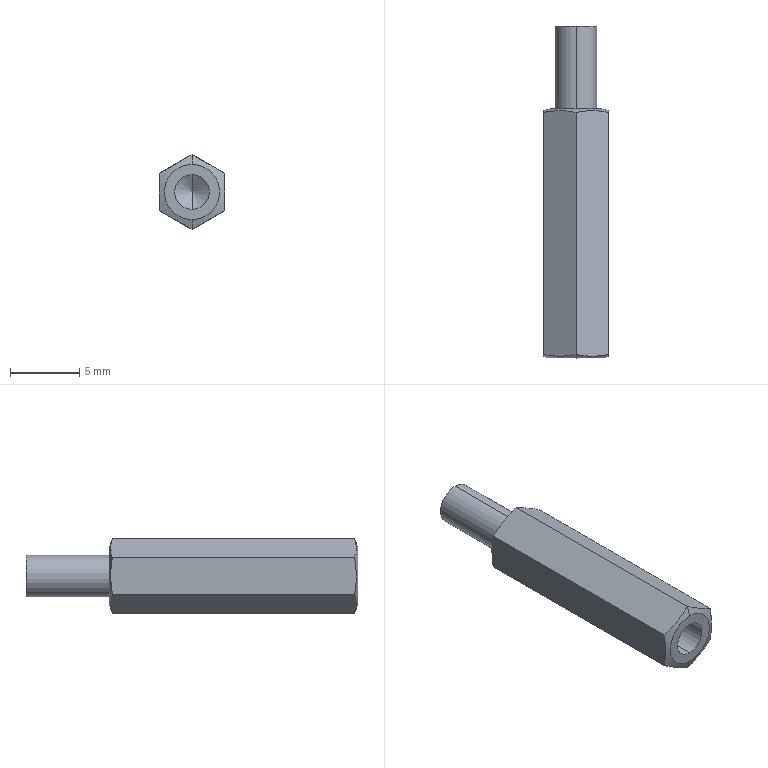Part | SolidWorks | features BaseBody 1 | 1 solid | 19 faces | box 4.7 x 24 x 5.427 mm | volume 364.722 mm3 | plane 9 | cone 6 | cylinder 4 | commonest cylinder face diameters 2.5 x2 3 x2
STEP:
#1=CARTESIAN_POINT('',(0.,0.,2.));
#2=VERTEX_POINT('',#1);
#3=CARTESIAN_POINT('',(0.,0.,-2.));
#4=VERTEX_POINT('',#3);
#5=CARTESIAN_POINT('',(0.,0.,0.));
#6=DIRECTION('',(0.,1.,0.));
#7=DIRECTION('',(0.,0.,1.));
#8=AXIS2_PLACEMENT_3D('',#5,#6,#7);
#9=CIRCLE('',#8,2.);
#10=EDGE_CURVE('',#2,#4,#9,.T.);
#11=ORIENTED_EDGE('',*,*,#10,.T.);
#12=CARTESIAN_POINT('',(0.,0.25,-2.714));
#13=VERTEX_POINT('',#12);
#14=CARTESIAN_POINT('',(0.,0.2515,-2.718));
#15=DIRECTION('',(0.,0.3307,-0.9438));
#16=VECTOR('',#15,1000.);
#17=LINE('',#14,#16);
#18=EDGE_CURVE('',#4,#13,#17,.T.);
#19=ORIENTED_EDGE('',*,*,#18,.T.);
#20=CARTESIAN_POINT('',(2.35,0.25,-1.357));
#21=VERTEX_POINT('',#20);
#22=CARTESIAN_POINT('',(0.,0.25,-2.714));
#23=CARTESIAN_POINT('',(0.3917,0.1708,-2.487));
#24=CARTESIAN_POINT('',(1.175,0.07448,-2.035));
#25=CARTESIAN_POINT('',(1.958,0.1708,-1.583));
#26=CARTESIAN_POINT('',(2.35,0.25,-1.357));
#27=B_SPLINE_CURVE_WITH_KNOTS('',3,(#22,#23,#24,#25,#26),.UNSPECIFIED.,.F.,.F.,(4,1,4),(0.,0.001357,0.002714),.UNSPECIFIED.);
#28=EDGE_CURVE('',#13,#21,#27,.T.);
#29=ORIENTED_EDGE('',*,*,#28,.T.);
#30=CARTESIAN_POINT('',(2.35,0.25,1.357));
#31=VERTEX_POINT('',#30);
#32=CARTESIAN_POINT('',(2.35,0.25,-1.357));
#33=CARTESIAN_POINT('',(2.35,0.1708,-0.9045));
#34=CARTESIAN_POINT('',(2.35,0.07448,-0.000000062));
#35=CARTESIAN_POINT('',(2.35,0.1708,0.9045));
#36=CARTESIAN_POINT('',(2.35,0.25,1.357));
#37=B_SPLINE_CURVE_WITH_KNOTS('',3,(#32,#33,#34,#35,#36),.UNSPECIFIED.,.F.,.F.,(4,1,4),(0.,0.001357,0.002714),.UNSPECIFIED.);
#38=EDGE_CURVE('',#21,#31,#37,.T.);
#39=ORIENTED_EDGE('',*,*,#38,.T.);
#40=CARTESIAN_POINT('',(0.,0.25,2.714));
#41=VERTEX_POINT('',#40);
#42=CARTESIAN_POINT('',(2.35,0.25,1.357));
#43=CARTESIAN_POINT('',(1.958,0.1708,1.583));
#44=CARTESIAN_POINT('',(1.175,0.07448,2.035));
#45=CARTESIAN_POINT('',(0.3917,0.1708,2.487));
#46=CARTESIAN_POINT('',(0.,0.25,2.714));
#47=B_SPLINE_CURVE_WITH_KNOTS('',3,(#42,#43,#44,#45,#46),.UNSPECIFIED.,.F.,.F.,(4,1,4),(0.,0.001357,0.002714),.UNSPECIFIED.);
#48=EDGE_CURVE('',#31,#41,#47,.T.);
#49=ORIENTED_EDGE('',*,*,#48,.T.);
#50=CARTESIAN_POINT('',(0.,0.2515,2.718));
#51=DIRECTION('',(0.,0.3307,0.9438));
#52=VECTOR('',#51,1000.);
#53=LINE('',#50,#52);
#54=EDGE_CURVE('',#2,#41,#53,.T.);
#55=ORIENTED_EDGE('',*,*,#54,.F.);
#56=EDGE_LOOP('',(#11,#19,#29,#39,#49,#55));
#57=FACE_OUTER_BOUND('',#56,.T.);
#58=CARTESIAN_POINT('',(0.,0.2515,0.));
#59=DIRECTION('',(0.,1.,0.));
#60=DIRECTION('',(0.,0.,1.));
#61=AXIS2_PLACEMENT_3D('',#58,#59,#60);
#62=CONICAL_SURFACE('',#61,2.718,1.234);
#63=ADVANCED_FACE('',(#57),#62,.T.);
#64=CARTESIAN_POINT('',(0.,18.,-2.));
#65=VERTEX_POINT('',#64);
#66=CARTESIAN_POINT('',(0.,18.,2.));
#67=VERTEX_POINT('',#66);
#68=CARTESIAN_POINT('',(0.,18.,0.));
#69=DIRECTION('',(0.,-1.,0.));
#70=DIRECTION('',(0.,0.,-1.));
#71=AXIS2_PLACEMENT_3D('',#68,#69,#70);
#72=CIRCLE('',#71,2.);
#73=EDGE_CURVE('',#65,#67,#72,.T.);
#74=ORIENTED_EDGE('',*,*,#73,.T.);
#75=CARTESIAN_POINT('',(0.,17.75,2.714));
#76=VERTEX_POINT('',#75);
#77=CARTESIAN_POINT('',(0.,17.749,2.718));
#78=DIRECTION('',(0.,-0.3307,0.9438));
#79=VECTOR('',#78,1000.);
#80=LINE('',#77,#79);
#81=EDGE_CURVE('',#67,#76,#80,.T.);
#82=ORIENTED_EDGE('',*,*,#81,.T.);
#83=CARTESIAN_POINT('',(2.35,17.75,1.357));
#84=VERTEX_POINT('',#83);
#85=CARTESIAN_POINT('',(0.,17.75,2.714));
#86=CARTESIAN_POINT('',(0.3917,17.829,2.487));
#87=CARTESIAN_POINT('',(1.175,17.926,2.035));
#88=CARTESIAN_POINT('',(1.958,17.829,1.583));
#89=CARTESIAN_POINT('',(2.35,17.75,1.357));
#90=B_SPLINE_CURVE_WITH_KNOTS('',3,(#85,#86,#87,#88,#89),.UNSPECIFIED.,.F.,.F.,(4,1,4),(0.,0.001357,0.002714),.UNSPECIFIED.);
#91=EDGE_CURVE('',#76,#84,#90,.T.);
#92=ORIENTED_EDGE('',*,*,#91,.T.);
#93=CARTESIAN_POINT('',(2.35,17.75,-1.357));
#94=VERTEX_POINT('',#93);
#95=CARTESIAN_POINT('',(2.35,17.75,1.357));
#96=CARTESIAN_POINT('',(2.35,17.829,0.9045));
#97=CARTESIAN_POINT('',(2.35,17.926,0.));
#98=CARTESIAN_POINT('',(2.35,17.829,-0.9045));
#99=CARTESIAN_POINT('',(2.35,17.75,-1.357));
#100=B_SPLINE_CURVE_WITH_KNOTS('',3,(#95,#96,#97,#98,#99),.UNSPECIFIED.,.F.,.F.,(4,1,4),(0.,0.001357,0.002714),.UNSPECIFIED.);
#101=EDGE_CURVE('',#84,#94,#100,.T.);
#102=ORIENTED_EDGE('',*,*,#101,.T.);
#103=CARTESIAN_POINT('',(0.,17.75,-2.714));
#104=VERTEX_POINT('',#103);
#105=CARTESIAN_POINT('',(2.35,17.75,-1.357));
#106=CARTESIAN_POINT('',(1.958,17.829,-1.583));
#107=CARTESIAN_POINT('',(1.175,17.926,-2.035));
#108=CARTESIAN_POINT('',(0.3917,17.829,-2.487));
#109=CARTESIAN_POINT('',(0.,17.75,-2.714));
#110=B_SPLINE_CURVE_WITH_KNOTS('',3,(#105,#106,#107,#108,#109),.UNSPECIFIED.,.F.,.F.,(4,1,4),(0.,0.001357,0.002714),.UNSPECIFIED.);
#111=EDGE_CURVE('',#94,#104,#110,.T.);
#112=ORIENTED_EDGE('',*,*,#111,.T.);
#113=CARTESIAN_POINT('',(0.,17.749,-2.718));
#114=DIRECTION('',(0.,-0.3307,-0.9438));
#115=VECTOR('',#114,1000.);
#116=LINE('',#113,#115);
#117=EDGE_CURVE('',#65,#104,#116,.T.);
#118=ORIENTED_EDGE('',*,*,#117,.F.);
#119=EDGE_LOOP('',(#74,#82,#92,#102,#112,#118));
#120=FACE_OUTER_BOUND('',#119,.T.);
#121=CARTESIAN_POINT('',(0.,17.749,0.));
#122=DIRECTION('',(0.,-1.,0.));
#123=DIRECTION('',(0.,0.,-1.));
#124=AXIS2_PLACEMENT_3D('',#121,#122,#123);
#125=CONICAL_SURFACE('',#124,2.718,1.234);
#126=ADVANCED_FACE('',(#120),#125,.T.);
#127=CARTESIAN_POINT('',(0.,4.,1.25));
#128=VERTEX_POINT('',#127);
#129=CARTESIAN_POINT('',(0.,4.,-1.25));
#130=VERTEX_POINT('',#129);
#131=CARTESIAN_POINT('',(0.,4.,0.));
#132=DIRECTION('',(0.,-1.,0.));
#133=DIRECTION('',(0.,0.,-1.));
#134=AXIS2_PLACEMENT_3D('',#131,#132,#133);
#135=CIRCLE('',#134,1.25);
#136=EDGE_CURVE('',#128,#130,#135,.T.);
#137=ORIENTED_EDGE('',*,*,#136,.F.);
#138=CARTESIAN_POINT('',(0.,0.,1.25));
#139=VERTEX_POINT('',#138);
#140=CARTESIAN_POINT('',(0.,0.,1.25));
#141=DIRECTION('',(0.,-1.,0.));
#142=VECTOR('',#141,1000.);
#143=LINE('',#140,#142);
#144=EDGE_CURVE('',#128,#139,#143,.T.);
#145=ORIENTED_EDGE('',*,*,#144,.T.);
#146=CARTESIAN_POINT('',(0.,0.,-1.25));
#147=VERTEX_POINT('',#146);
#148=CARTESIAN_POINT('',(0.,0.,0.));
#149=DIRECTION('',(0.,-1.,0.));
#150=DIRECTION('',(0.,0.,-1.));
#151=AXIS2_PLACEMENT_3D('',#148,#149,#150);
#152=CIRCLE('',#151,1.25);
#153=EDGE_CURVE('',#139,#147,#152,.T.);
#154=ORIENTED_EDGE('',*,*,#153,.T.);
#155=CARTESIAN_POINT('',(0.,0.,-1.25));
#156=DIRECTION('',(0.,-1.,0.));
#157=VECTOR('',#156,1000.);
#158=LINE('',#155,#157);
#159=EDGE_CURVE('',#130,#147,#158,.T.);
#160=ORIENTED_EDGE('',*,*,#159,.F.);
#161=EDGE_LOOP('',(#137,#145,#154,#160));
#162=FACE_OUTER_BOUND('',#161,.T.);
#163=CARTESIAN_POINT('',(0.,0.,0.));
#164=DIRECTION('',(0.,-1.,0.));
#165=DIRECTION('',(0.,0.,-1.));
#166=AXIS2_PLACEMENT_3D('',#163,#164,#165);
#167=CYLINDRICAL_SURFACE('',#166,1.25);
#168=ADVANCED_FACE('',(#162),#167,.F.);
#169=CARTESIAN_POINT('',(0.,24.,-1.5));
#170=VERTEX_POINT('',#169);
#171=CARTESIAN_POINT('',(0.,24.,1.5));
#172=VERTEX_POINT('',#171);
#173=CARTESIAN_POINT('',(0.,24.,0.));
#174=DIRECTION('',(0.,-1.,0.));
#175=DIRECTION('',(0.,0.,-1.));
#176=AXIS2_PLACEMENT_3D('',#173,#174,#175);
#177=CIRCLE('',#176,1.5);
#178=EDGE_CURVE('',#170,#172,#177,.T.);
#179=ORIENTED_EDGE('',*,*,#178,.T.);
#180=CARTESIAN_POINT('',(0.,18.,1.5));
#181=VERTEX_POINT('',#180);
#182=CARTESIAN_POINT('',(0.,24.,1.5));
#183=DIRECTION('',(0.,-1.,0.));
#184=VECTOR('',#183,1000.);
#185=LINE('',#182,#184);
#186=EDGE_CURVE('',#172,#181,#185,.T.);
#187=ORIENTED_EDGE('',*,*,#186,.T.);
#188=CARTESIAN_POINT('',(0.,18.,-1.5));
#189=VERTEX_POINT('',#188);
#190=CARTESIAN_POINT('',(0.,18.,0.));
#191=DIRECTION('',(0.,-1.,0.));
#192=DIRECTION('',(0.,0.,-1.));
#193=AXIS2_PLACEMENT_3D('',#190,#191,#192);
#194=CIRCLE('',#193,1.5);
#195=EDGE_CURVE('',#189,#181,#194,.T.);
#196=ORIENTED_EDGE('',*,*,#195,.F.);
#197=CARTESIAN_POINT('',(0.,24.,-1.5));
#198=DIRECTION('',(0.,-1.,0.));
#199=VECTOR('',#198,1000.);
#200=LINE('',#197,#199);
#201=EDGE_CURVE('',#170,#189,#200,.T.);
#202=ORIENTED_EDGE('',*,*,#201,.F.);
#203=EDGE_LOOP('',(#179,#187,#196,#202));
#204=FACE_OUTER_BOUND('',#203,.T.);
#205=CARTESIAN_POINT('',(0.,24.,0.));
#206=DIRECTION('',(0.,-1.,0.));
#207=DIRECTION('',(0.,0.,-1.));
#208=AXIS2_PLACEMENT_3D('',#205,#206,#207);
#209=CYLINDRICAL_SURFACE('',#208,1.5);
#210=ADVANCED_FACE('',(#204),#209,.T.);
#211=CARTESIAN_POINT('',(0.,4.751,0.));
#212=VERTEX_POINT('',#211);
#213=CARTESIAN_POINT('',(0.,4.,-1.25));
#214=DIRECTION('',(0.,-0.515,-0.8572));
#215=VECTOR('',#214,1000.);
#216=LINE('',#213,#215);
#217=EDGE_CURVE('',#212,#130,#216,.T.);
#218=ORIENTED_EDGE('',*,*,#217,.F.);
#219=CARTESIAN_POINT('',(0.,4.,1.25));
#220=DIRECTION('',(0.,-0.515,0.8572));
#221=VECTOR('',#220,1000.);
#222=LINE('',#219,#221);
#223=EDGE_CURVE('',#212,#128,#222,.T.);
#224=ORIENTED_EDGE('',*,*,#223,.T.);
#225=ORIENTED_EDGE('',*,*,#136,.T.);
#226=EDGE_LOOP('',(#218,#224,#225));
#227=FACE_OUTER_BOUND('',#226,.T.);
#228=CARTESIAN_POINT('',(0.,4.,0.));
#229=DIRECTION('',(0.,-1.,0.));
#230=DIRECTION('',(0.,0.,-1.));
#231=AXIS2_PLACEMENT_3D('',#228,#229,#230);
#232=CONICAL_SURFACE('',#231,1.25,1.03);
#233=ADVANCED_FACE('',(#227),#232,.F.);
#234=CARTESIAN_POINT('',(2.35,18.,1.357));
#235=DIRECTION('',(0.,-1.,0.));
#236=VECTOR('',#235,1000.);
#237=LINE('',#234,#236);
#238=EDGE_CURVE('',#84,#31,#237,.T.);
#239=ORIENTED_EDGE('',*,*,#238,.F.);
#240=ORIENTED_EDGE('',*,*,#91,.F.);
#241=CARTESIAN_POINT('',(0.,18.,2.714));
#242=DIRECTION('',(0.,1.,0.));
#243=VECTOR('',#242,1000.);
#244=LINE('',#241,#243);
#245=EDGE_CURVE('',#41,#76,#244,.T.);
#246=ORIENTED_EDGE('',*,*,#245,.F.);
#247=ORIENTED_EDGE('',*,*,#48,.F.);
#248=EDGE_LOOP('',(#239,#240,#246,#247));
#249=FACE_OUTER_BOUND('',#248,.T.);
#250=CARTESIAN_POINT('',(0.,18.,2.714));
#251=DIRECTION('',(-0.5,0.,-0.866));
#252=DIRECTION('',(-0.866,0.,0.5));
#253=AXIS2_PLACEMENT_3D('',#250,#251,#252);
#254=PLANE('',#253);
#255=ADVANCED_FACE('',(#249),#254,.F.);
#256=ORIENTED_EDGE('',*,*,#18,.F.);
#257=CARTESIAN_POINT('',(0.,0.,0.));
#258=DIRECTION('',(0.,1.,0.));
#259=DIRECTION('',(0.,0.,1.));
#260=AXIS2_PLACEMENT_3D('',#257,#258,#259);
#261=CIRCLE('',#260,2.);
#262=EDGE_CURVE('',#4,#2,#261,.T.);
#263=ORIENTED_EDGE('',*,*,#262,.T.);
#264=ORIENTED_EDGE('',*,*,#54,.T.);
#265=CARTESIAN_POINT('',(-2.35,0.25,1.357));
#266=VERTEX_POINT('',#265);
#267=CARTESIAN_POINT('',(0.,0.25,2.714));
#268=CARTESIAN_POINT('',(-0.3917,0.1708,2.487));
#269=CARTESIAN_POINT('',(-1.175,0.07448,2.035));
#270=CARTESIAN_POINT('',(-1.958,0.1708,1.583));
#271=CARTESIAN_POINT('',(-2.35,0.25,1.357));
#272=B_SPLINE_CURVE_WITH_KNOTS('',3,(#267,#268,#269,#270,#271),.UNSPECIFIED.,.F.,.F.,(4,1,4),(0.,0.001357,0.002714),.UNSPECIFIED.);
#273=EDGE_CURVE('',#41,#266,#272,.T.);
#274=ORIENTED_EDGE('',*,*,#273,.T.);
#275=CARTESIAN_POINT('',(-2.35,0.25,-1.357));
#276=VERTEX_POINT('',#275);
#277=CARTESIAN_POINT('',(-2.35,0.25,1.357));
#278=CARTESIAN_POINT('',(-2.35,0.1708,0.9045));
#279=CARTESIAN_POINT('',(-2.35,0.07448,0.000000048));
#280=CARTESIAN_POINT('',(-2.35,0.1708,-0.9045));
#281=CARTESIAN_POINT('',(-2.35,0.25,-1.357));
#282=B_SPLINE_CURVE_WITH_KNOTS('',3,(#277,#278,#279,#280,#281),.UNSPECIFIED.,.F.,.F.,(4,1,4),(0.,0.001357,0.002714),.UNSPECIFIED.);
#283=EDGE_CURVE('',#266,#276,#282,.T.);
#284=ORIENTED_EDGE('',*,*,#283,.T.);
#285=CARTESIAN_POINT('',(-2.35,0.25,-1.357));
#286=CARTESIAN_POINT('',(-1.958,0.1708,-1.583));
#287=CARTESIAN_POINT('',(-1.175,0.07448,-2.035));
#288=CARTESIAN_POINT('',(-0.3917,0.1708,-2.487));
#289=CARTESIAN_POINT('',(0.,0.25,-2.714));
#290=B_SPLINE_CURVE_WITH_KNOTS('',3,(#285,#286,#287,#288,#289),.UNSPECIFIED.,.F.,.F.,(4,1,4),(0.,0.001357,0.002714),.UNSPECIFIED.);
#291=EDGE_CURVE('',#276,#13,#290,.T.);
#292=ORIENTED_EDGE('',*,*,#291,.T.);
#293=EDGE_LOOP('',(#256,#263,#264,#274,#284,#292));
#294=FACE_OUTER_BOUND('',#293,.T.);
#295=CARTESIAN_POINT('',(0.,0.2515,0.));
#296=DIRECTION('',(0.,1.,0.));
#297=DIRECTION('',(0.,0.,1.));
#298=AXIS2_PLACEMENT_3D('',#295,#296,#297);
#299=CONICAL_SURFACE('',#298,2.718,1.234);
#300=ADVANCED_FACE('',(#294),#299,.T.);
#301=CARTESIAN_POINT('',(2.35,18.,-1.357));
#302=DIRECTION('',(0.,-1.,0.));
#303=VECTOR('',#302,1000.);
#304=LINE('',#301,#303);
#305=EDGE_CURVE('',#94,#21,#304,.T.);
#306=ORIENTED_EDGE('',*,*,#305,.F.);
#307=ORIENTED_EDGE('',*,*,#101,.F.);
#308=ORIENTED_EDGE('',*,*,#238,.T.);
#309=ORIENTED_EDGE('',*,*,#38,.F.);
#310=EDGE_LOOP('',(#306,#307,#308,#309));
#311=FACE_OUTER_BOUND('',#310,.T.);
#312=CARTESIAN_POINT('',(2.35,18.,1.357));
#313=DIRECTION('',(-1.,0.,0.));
#314=DIRECTION('',(0.,0.,1.));
#315=AXIS2_PLACEMENT_3D('',#312,#313,#314);
#316=PLANE('',#315);
#317=ADVANCED_FACE('',(#311),#316,.F.);
#318=ORIENTED_EDGE('',*,*,#81,.F.);
#319=CARTESIAN_POINT('',(0.,18.,0.));
#320=DIRECTION('',(0.,-1.,0.));
#321=DIRECTION('',(0.,0.,-1.));
#322=AXIS2_PLACEMENT_3D('',#319,#320,#321);
#323=CIRCLE('',#322,2.);
#324=EDGE_CURVE('',#67,#65,#323,.T.);
#325=ORIENTED_EDGE('',*,*,#324,.T.);
#326=ORIENTED_EDGE('',*,*,#117,.T.);
#327=CARTESIAN_POINT('',(-2.35,17.75,-1.357));
#328=VERTEX_POINT('',#327);
#329=CARTESIAN_POINT('',(0.,17.75,-2.714));
#330=CARTESIAN_POINT('',(-0.3917,17.829,-2.487));
#331=CARTESIAN_POINT('',(-1.175,17.926,-2.035));
#332=CARTESIAN_POINT('',(-1.958,17.829,-1.583));
#333=CARTESIAN_POINT('',(-2.35,17.75,-1.357));
#334=B_SPLINE_CURVE_WITH_KNOTS('',3,(#329,#330,#331,#332,#333),.UNSPECIFIED.,.F.,.F.,(4,1,4),(0.,0.001357,0.002714),.UNSPECIFIED.);
#335=EDGE_CURVE('',#104,#328,#334,.T.);
#336=ORIENTED_EDGE('',*,*,#335,.T.);
#337=CARTESIAN_POINT('',(-2.35,17.75,1.357));
#338=VERTEX_POINT('',#337);
#339=CARTESIAN_POINT('',(-2.35,17.75,-1.357));
#340=CARTESIAN_POINT('',(-2.35,17.829,-0.9045));
#341=CARTESIAN_POINT('',(-2.35,17.926,-0.000000061));
#342=CARTESIAN_POINT('',(-2.35,17.829,0.9045));
#343=CARTESIAN_POINT('',(-2.35,17.75,1.357));
#344=B_SPLINE_CURVE_WITH_KNOTS('',3,(#339,#340,#341,#342,#343),.UNSPECIFIED.,.F.,.F.,(4,1,4),(0.,0.001357,0.002714),.UNSPECIFIED.);
#345=EDGE_CURVE('',#328,#338,#344,.T.);
#346=ORIENTED_EDGE('',*,*,#345,.T.);
#347=CARTESIAN_POINT('',(-2.35,17.75,1.357));
#348=CARTESIAN_POINT('',(-1.958,17.829,1.583));
#349=CARTESIAN_POINT('',(-1.175,17.926,2.035));
#350=CARTESIAN_POINT('',(-0.3917,17.829,2.487));
#351=CARTESIAN_POINT('',(0.,17.75,2.714));
#352=B_SPLINE_CURVE_WITH_KNOTS('',3,(#347,#348,#349,#350,#351),.UNSPECIFIED.,.F.,.F.,(4,1,4),(0.,0.001357,0.002714),.UNSPECIFIED.);
#353=EDGE_CURVE('',#338,#76,#352,.T.);
#354=ORIENTED_EDGE('',*,*,#353,.T.);
#355=EDGE_LOOP('',(#318,#325,#326,#336,#346,#354));
#356=FACE_OUTER_BOUND('',#355,.T.);
#357=CARTESIAN_POINT('',(0.,17.749,0.));
#358=DIRECTION('',(0.,-1.,0.));
#359=DIRECTION('',(0.,0.,-1.));
#360=AXIS2_PLACEMENT_3D('',#357,#358,#359);
#361=CONICAL_SURFACE('',#360,2.718,1.234);
#362=ADVANCED_FACE('',(#356),#361,.T.);
#363=ORIENTED_EDGE('',*,*,#245,.T.);
#364=ORIENTED_EDGE('',*,*,#353,.F.);
#365=CARTESIAN_POINT('',(-2.35,18.,1.357));
#366=DIRECTION('',(0.,1.,0.));
#367=VECTOR('',#366,1000.);
#368=LINE('',#365,#367);
#369=EDGE_CURVE('',#266,#338,#368,.T.);
#370=ORIENTED_EDGE('',*,*,#369,.F.);
#371=ORIENTED_EDGE('',*,*,#273,.F.);
#372=EDGE_LOOP('',(#363,#364,#370,#371));
#373=FACE_OUTER_BOUND('',#372,.T.);
#374=CARTESIAN_POINT('',(-2.35,18.,1.357));
#375=DIRECTION('',(0.5,0.,-0.866));
#376=DIRECTION('',(-0.866,0.,-0.5));
#377=AXIS2_PLACEMENT_3D('',#374,#375,#376);
#378=PLANE('',#377);
#379=ADVANCED_FACE('',(#373),#378,.F.);
#380=CARTESIAN_POINT('',(0.,18.,-2.714));
#381=DIRECTION('',(0.,-1.,0.));
#382=VECTOR('',#381,1000.);
#383=LINE('',#380,#382);
#384=EDGE_CURVE('',#104,#13,#383,.T.);
#385=ORIENTED_EDGE('',*,*,#384,.F.);
#386=ORIENTED_EDGE('',*,*,#111,.F.);
#387=ORIENTED_EDGE('',*,*,#305,.T.);
#388=ORIENTED_EDGE('',*,*,#28,.F.);
#389=EDGE_LOOP('',(#385,#386,#387,#388));
#390=FACE_OUTER_BOUND('',#389,.T.);
#391=CARTESIAN_POINT('',(2.35,18.,-1.357));
#392=DIRECTION('',(-0.5,0.,0.866));
#393=DIRECTION('',(0.866,0.,0.5));
#394=AXIS2_PLACEMENT_3D('',#391,#392,#393);
#395=PLANE('',#394);
#396=ADVANCED_FACE('',(#390),#395,.F.);
#397=ORIENTED_EDGE('',*,*,#10,.F.);
#398=ORIENTED_EDGE('',*,*,#262,.F.);
#399=EDGE_LOOP('',(#397,#398));
#400=FACE_OUTER_BOUND('',#399,.T.);
#401=CARTESIAN_POINT('',(0.,0.,0.));
#402=DIRECTION('',(0.,-1.,0.));
#403=DIRECTION('',(0.,0.,-1.));
#404=AXIS2_PLACEMENT_3D('',#401,#402,#403);
#405=CIRCLE('',#404,1.25);
#406=EDGE_CURVE('',#147,#139,#405,.T.);
#407=ORIENTED_EDGE('',*,*,#406,.F.);
#408=ORIENTED_EDGE('',*,*,#153,.F.);
#409=EDGE_LOOP('',(#407,#408));
#410=FACE_BOUND('',#409,.T.);
#411=CARTESIAN_POINT('',(0.,0.,0.));
#412=DIRECTION('',(0.,1.,0.));
#413=DIRECTION('',(0.,0.,1.));
#414=AXIS2_PLACEMENT_3D('',#411,#412,#413);
#415=PLANE('',#414);
#416=ADVANCED_FACE('',(#400,#410),#415,.F.);
#417=ORIENTED_EDGE('',*,*,#73,.F.);
#418=ORIENTED_EDGE('',*,*,#324,.F.);
#419=EDGE_LOOP('',(#417,#418));
#420=FACE_OUTER_BOUND('',#419,.T.);
#421=ORIENTED_EDGE('',*,*,#195,.T.);
#422=CARTESIAN_POINT('',(0.,18.,0.));
#423=DIRECTION('',(0.,-1.,0.));
#424=DIRECTION('',(0.,0.,-1.));
#425=AXIS2_PLACEMENT_3D('',#422,#423,#424);
#426=CIRCLE('',#425,1.5);
#427=EDGE_CURVE('',#181,#189,#426,.T.);
#428=ORIENTED_EDGE('',*,*,#427,.T.);
#429=EDGE_LOOP('',(#421,#428));
#430=FACE_BOUND('',#429,.T.);
#431=CARTESIAN_POINT('',(0.,18.,0.));
#432=DIRECTION('',(0.,1.,0.));
#433=DIRECTION('',(0.,0.,1.));
#434=AXIS2_PLACEMENT_3D('',#431,#432,#433);
#435=PLANE('',#434);
#436=ADVANCED_FACE('',(#420,#430),#435,.T.);
#437=ORIENTED_EDGE('',*,*,#369,.T.);
#438=ORIENTED_EDGE('',*,*,#345,.F.);
#439=CARTESIAN_POINT('',(-2.35,18.,-1.357));
#440=DIRECTION('',(0.,1.,0.));
#441=VECTOR('',#440,1000.);
#442=LINE('',#439,#441);
#443=EDGE_CURVE('',#276,#328,#442,.T.);
#444=ORIENTED_EDGE('',*,*,#443,.F.);
#445=ORIENTED_EDGE('',*,*,#283,.F.);
#446=EDGE_LOOP('',(#437,#438,#444,#445));
#447=FACE_OUTER_BOUND('',#446,.T.);
#448=CARTESIAN_POINT('',(-2.35,18.,-1.357));
#449=DIRECTION('',(1.,0.,0.));
#450=DIRECTION('',(0.,0.,-1.));
#451=AXIS2_PLACEMENT_3D('',#448,#449,#450);
#452=PLANE('',#451);
#453=ADVANCED_FACE('',(#447),#452,.F.);
#454=ORIENTED_EDGE('',*,*,#443,.T.);
#455=ORIENTED_EDGE('',*,*,#335,.F.);
#456=ORIENTED_EDGE('',*,*,#384,.T.);
#457=ORIENTED_EDGE('',*,*,#291,.F.);
#458=EDGE_LOOP('',(#454,#455,#456,#457));
#459=FACE_OUTER_BOUND('',#458,.T.);
#460=CARTESIAN_POINT('',(0.,18.,-2.714));
#461=DIRECTION('',(0.5,0.,0.866));
#462=DIRECTION('',(0.866,0.,-0.5));
#463=AXIS2_PLACEMENT_3D('',#460,#461,#462);
#464=PLANE('',#463);
#465=ADVANCED_FACE('',(#459),#464,.F.);
#466=ORIENTED_EDGE('',*,*,#144,.F.);
#467=CARTESIAN_POINT('',(0.,4.,0.));
#468=DIRECTION('',(0.,-1.,0.));
#469=DIRECTION('',(0.,0.,-1.));
#470=AXIS2_PLACEMENT_3D('',#467,#468,#469);
#471=CIRCLE('',#470,1.25);
#472=EDGE_CURVE('',#130,#128,#471,.T.);
#473=ORIENTED_EDGE('',*,*,#472,.F.);
#474=ORIENTED_EDGE('',*,*,#159,.T.);
#475=ORIENTED_EDGE('',*,*,#406,.T.);
#476=EDGE_LOOP('',(#466,#473,#474,#475));
#477=FACE_OUTER_BOUND('',#476,.T.);
#478=CARTESIAN_POINT('',(0.,0.,0.));
#479=DIRECTION('',(0.,-1.,0.));
#480=DIRECTION('',(0.,0.,-1.));
#481=AXIS2_PLACEMENT_3D('',#478,#479,#480);
#482=CYLINDRICAL_SURFACE('',#481,1.25);
#483=ADVANCED_FACE('',(#477),#482,.F.);
#484=ORIENTED_EDGE('',*,*,#186,.F.);
#485=CARTESIAN_POINT('',(0.,24.,0.));
#486=DIRECTION('',(0.,-1.,0.));
#487=DIRECTION('',(0.,0.,-1.));
#488=AXIS2_PLACEMENT_3D('',#485,#486,#487);
#489=CIRCLE('',#488,1.5);
#490=EDGE_CURVE('',#172,#170,#489,.T.);
#491=ORIENTED_EDGE('',*,*,#490,.T.);
#492=ORIENTED_EDGE('',*,*,#201,.T.);
#493=ORIENTED_EDGE('',*,*,#427,.F.);
#494=EDGE_LOOP('',(#484,#491,#492,#493));
#495=FACE_OUTER_BOUND('',#494,.T.);
#496=CARTESIAN_POINT('',(0.,24.,0.));
#497=DIRECTION('',(0.,-1.,0.));
#498=DIRECTION('',(0.,0.,-1.));
#499=AXIS2_PLACEMENT_3D('',#496,#497,#498);
#500=CYLINDRICAL_SURFACE('',#499,1.5);
#501=ADVANCED_FACE('',(#495),#500,.T.);
#502=ORIENTED_EDGE('',*,*,#223,.F.);
#503=ORIENTED_EDGE('',*,*,#217,.T.);
#504=ORIENTED_EDGE('',*,*,#472,.T.);
#505=EDGE_LOOP('',(#502,#503,#504));
#506=FACE_OUTER_BOUND('',#505,.T.);
#507=CARTESIAN_POINT('',(0.,4.,0.));
#508=DIRECTION('',(0.,-1.,0.));
#509=DIRECTION('',(0.,0.,-1.));
#510=AXIS2_PLACEMENT_3D('',#507,#508,#509);
#511=CONICAL_SURFACE('',#510,1.25,1.03);
#512=ADVANCED_FACE('',(#506),#511,.F.);
#513=ORIENTED_EDGE('',*,*,#178,.F.);
#514=ORIENTED_EDGE('',*,*,#490,.F.);
#515=EDGE_LOOP('',(#513,#514));
#516=FACE_OUTER_BOUND('',#515,.T.);
#517=CARTESIAN_POINT('',(0.,24.,0.));
#518=DIRECTION('',(0.,1.,0.));
#519=DIRECTION('',(0.,0.,1.));
#520=AXIS2_PLACEMENT_3D('',#517,#518,#519);
#521=PLANE('',#520);
#522=ADVANCED_FACE('',(#516),#521,.T.);
#523=CLOSED_SHELL('',(#63,#126,#168,#210,#233,#255,#300,#317,#362,#379,#396,#416,#436,#453,#465,#483,#501,#512,#522));
#524=MANIFOLD_SOLID_BREP('',#523);
#525=CARTESIAN_POINT('',(0.,0.,0.));
#526=DIRECTION('',(0.,0.,1.));
#527=DIRECTION('',(1.,0.,0.));
#528=AXIS2_PLACEMENT_3D('',#525,#526,#527);
#529=(LENGTH_UNIT()NAMED_UNIT(*)SI_UNIT(.MILLI.,.METRE.));
#530=UNCERTAINTY_MEASURE_WITH_UNIT(LENGTH_MEASURE(0.00001),#529,'','');
#531=(NAMED_UNIT(*)PLANE_ANGLE_UNIT()SI_UNIT($,.RADIAN.));
#532=(NAMED_UNIT(*)SI_UNIT($,.STERADIAN.)SOLID_ANGLE_UNIT());
#533=(GEOMETRIC_REPRESENTATION_CONTEXT(3)GLOBAL_UNCERTAINTY_ASSIGNED_CONTEXT((#530))GLOBAL_UNIT_ASSIGNED_CONTEXT((#529,#531,#532))REPRESENTATION_CONTEXT('',''));
#534=ADVANCED_BREP_SHAPE_REPRESENTATION('',(#524,#528),#533);